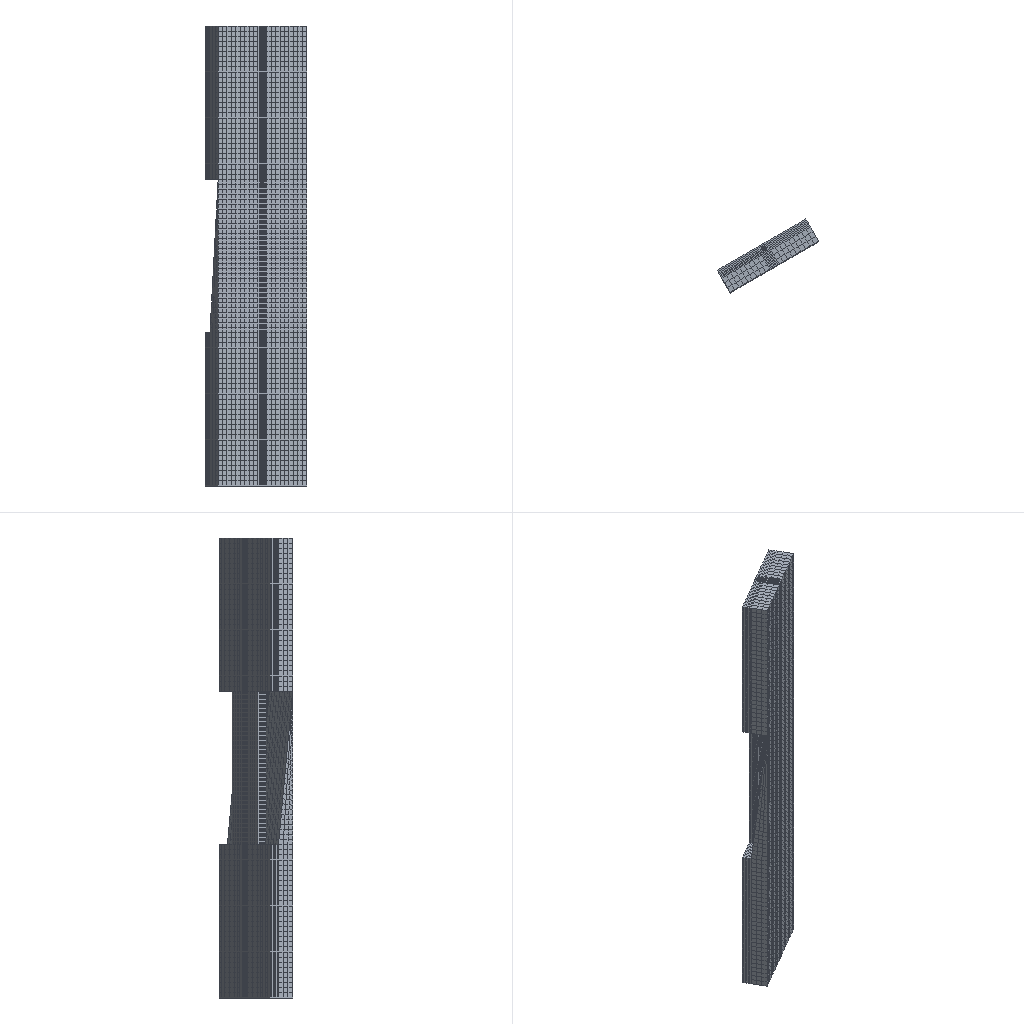Simulation study | abaqus
Set-up summary:
category,name,step,type,value,unit,region
solver,abaqus
solver,version,,,Abaqus/Standard 2020
units,not stated in the deck,,not stated
analysis,deck,,transient,transient
load_step,step,step,transient
load_step,requested,,,1
mesh,nodes,,,35012
mesh,elements,,,27514
element_type,C3D8,,solid,27514
load,load commands in deck,,count,3
bc,support commands in deck,,count,13
material,MAT-HUACHUANG,,in results
material,MAT-PIPE,,in results
material,MATE-HUATI,,in results
check,setup vs results,,match,"per instance, exact: element labels, types and connectivity; labels of the nodes the elements use; coordinates of those nodes at SINGLE_PRECISION in 3 of 3 instance(s)"
Abaqus input file, long lists of numbers shortened:
*Heading
** Job name: Job-2 Model name: Model-1
** Generated by: Abaqus/CAE 2020
*Preprint, echo=NO, model=NO, history=NO, contact=NO
**
** PARTS
**
*Part, name=huachuang
*Node
      1,           5.,   7.59,         120.
      2,           5.,   7.59,         180.
** (21850 more lines like these left out)
*Element, type=C3D8
  1,  2430,  2431, 12315, 12228,    96,    97,  2257,  2256
  2,  2431,  2432, 12316, 12315,    97,    98,  2258,  2257
** (17672 more lines like these left out)
*Nset, nset=Set-9, generate
     1,  21852,      1
*Elset, elset=Set-9, generate
     1,  17674,      1
*Elset, elset=_Surf-huachuang_S4, internal
 9200, 9203, 9206, 9209, 9212, 9215, 9218, 9221, 9224, 9227, 9230, 9233, 9236, 9239, 9242, 9245
 9248, 9251, 9254, 9257, 9260, 9263, 9266, 9269, 9272, 9275, 9278, 9281, 9284, 9287, 9500, 9503
** (1 more lines like these left out)
*Elset, elset=_Surf-huachuang_S3, internal
 9288, 9289, 9290, 9291, 9292, 9293, 9294, 9295, 9296, 9297, 9298, 9299, 9300, 9301, 9302, 9333
 9334, 9335, 9336, 9337, 9338, 9339, 9340, 9341, 9342, 9343, 9344, 9345, 9346, 9347, 9543, 9544
** (1 more lines like these left out)
*Elset, elset=_Surf-huachuang_S2, internal
  4938,  4939,  4940,  4941,  4942,  4943,  4944,  4945,  4946,  4947,  4948,  4949,  4950,  4951,  4952,  4953
  4954,  4955,  4956,  4957,  4958,  4959,  4960,  4961,  4962,  4963,  4964,  4965,  4966,  4967,  4968,  4969
** (15 more lines like these left out)
*Elset, elset=_Surf-huachuang_S5, internal
 12494, 12495, 12496, 12497, 12498, 12499, 12500, 12501, 12502, 12503, 12504, 12505, 12506, 12507, 12508, 12509
 12510, 12511, 12512, 12513, 12514, 12515, 12516, 12517, 12518, 12519, 12520, 12521, 12522, 12523, 12614, 12615
** (15 more lines like these left out)
*Surface, type=ELEMENT, name=Surf-huachuang
_Surf-huachuang_S4, S4
_Surf-huachuang_S3, S3
_Surf-huachuang_S2, S2
_Surf-huachuang_S5, S5
** Section: Section-huachuang
*Solid Section, elset=Set-9, material=Mat-huachuang
,
*End Part
**
*Part, name=huati
*Node
      1,           7.,          10.,         120.
      2,           7.,   8.2,         120.
** (11222 more lines like these left out)
*Element, type=C3D8
  1, 1393, 1394, 6416, 6387,   66,   67, 1268, 1267
  2, 1394, 1395, 6415, 6416,   67,   68, 1269, 1268
** (8878 more lines like these left out)
*Nset, nset=Set-23, generate
     1,  11224,      1
*Elset, elset=Set-23, generate
    1,  8880,     1
** Section: Section-huati
*Solid Section, elset=Set-23, material=Mate-huati
,
*End Part
**
*Part, name=pipe
*Node
      1,  0.5911,           0.,           0.
      2,  0.5911,           0.,         180.
** (1934 more lines like these left out)
*Element, type=C3D8
  1,    8,  377, 1104,  498,    1,   19,  985,  258
  2,  377,  376, 1105, 1104,   19,   20,  986,  985
** (958 more lines like these left out)
*Nset, nset=Set-pipe, generate
    1,  1936,     1
*Elset, elset=Set-pipe, generate
   1,  960,    1
** Section: Section-pipe
*Solid Section, elset=Set-pipe, material=Mat-pipe
,
*End Part
**
**
** ASSEMBLY
**
*Assembly, name=Assembly
**
*Instance, name=huachuang-1, part=huachuang
          0.,           0.,           0.
          0.,           0.,           0.,           0.,           0., 1., 30.
*End Instance
**
*Instance, name=pipe-1, part=pipe
0.2301, 9.601,           0.
0.2301, 9.601,           0., 0.2301, 9.601, 1., 30.
*End Instance
**
*Instance, name=huati-1, part=huati
          0.,           0.,           0.
          0.,           0.,           0.,           0.,           0., 1., 30.
*End Instance
**
*Nset, nset=Set-9, instance=pipe-1, generate
    1,  1936,     1
*Elset, elset=Set-9, instance=pipe-1, generate
   1,  960,    1
*Nset, nset=Set-Huati, instance=huati-1, generate
     1,  11224,      1
*Elset, elset=Set-Huati, instance=huati-1, generate
    1,  8880,     1
*Nset, nset=Set-Huati-Side, instance=huati-1
    1,    2,    3,    4,    5,    6,    7,    8,    9,   10,   11,   12,   13,   14,   15,   16
   17,   18,   19,   20,   21,   22,   23,   24,   25,   26,   27,   28,   29,   30,   31,   32
** (21 more lines like these left out)
*Elset, elset=Set-Huati-Side, instance=huati-1
   30,   31,   32,  120,  150,  151,  181,  182,  183,  271,  272,  273,  274,  275,  276,  451
  452,  453,  454,  571,  572,  573,  661,  662,  663,  664,  781,  782,  783,  784,  785,  786
** (17 more lines like these left out)
*Nset, nset=Set-cemian, instance=huachuang-1
     2,     3,     5,     8,    10,    12,    14,    19,    20,    21,    22,    23,    25,    27,    31,    32
    34,    37,    38,    40,    43,    44,    46,    48,    51,    52,    54,    55,    59,    60,    64,    65
** (36 more lines like these left out)
*Nset, nset=Set-cemian, instance=pipe-1
   1,   2,   3,   4,   5,   6,   7,   8,   9,  10,  11,  12,  13,  14,  15,  16
  17,  18, 138, 258, 378, 498, 618, 619, 739, 740, 741, 861, 862, 982, 983, 984
*Elset, elset=Set-cemian, instance=huachuang-1
   105,   120,   135,   150,   165,   180,   181,   182,   211,   212,   315,   330,   345,   420,   465,   480
   568,   569,   570,   658,   659,   660,   748,   749,   750,   838,   839,   840,  1284,  1285,  1286,  1374
** (30 more lines like these left out)
*Elset, elset=Set-cemian, instance=pipe-1
   1, 120, 121, 240, 241, 360, 361, 480, 481, 600, 601, 720, 721, 840, 841, 960
*Nset, nset=Set-dimian, instance=huachuang-1
    11,    12,    13,    14,    16,    18,    19,    21,    39,    40,    42,    43,    53,    54,    70,    71
    80,    81,    88,    89,   270,   271,   272,   273,   274,   275,   276,   277,   278,   279,   280,   281
** (154 more lines like these left out)
*Elset, elset=Set-dimian, instance=huachuang-1
   481,   484,   487,   490,   493,   496,   499,   502,   505,   508,   511,   514,   517,   520,   523,   526
   529,   532,   535,   538,   541,   544,   547,   550,   553,   556,   559,   562,   565,   568,   571,   574
** (146 more lines like these left out)
*Nset, nset=Set-load, instance=huati-1
   11,   12,   15,   16,   35,   36,  358,  359,  360,  361,  362,  363,  364,  365,  366,  367
  368,  369,  370,  371,  372,  373,  374,  375,  376,  377,  378,  379,  380,  381,  382,  383
** (29 more lines like these left out)
*Elset, elset=Set-load, instance=huati-1
  961,  962,  963,  964,  965,  966,  967,  968,  969,  970,  971,  972,  973,  974,  975,  976
  977,  978,  979,  980,  981,  982,  983,  984,  985,  986,  987,  988,  989,  990,  991,  992
** (25 more lines like these left out)
*Nset, nset=Set-qianmian, instance=huachuang-1
    35,    36,    37,    38,    39,    40,    41,    42,    43,    44,    45,    46,    47,    48,    50,    52
    78,    79,    80,    81,    82,    83,    84,    85,    86,    87,    88,    89,    90,    91,    92,    93
** (93 more lines like these left out)
*Elset, elset=Set-qianmian, instance=huachuang-1
  2517,  2518,  2519,  2520,  2521,  2522,  2523,  2524,  2525,  2526,  2527,  2528,  2529,  2530,  2531,  2532
  2533,  2534,  2535,  2536,  2537,  2538,  2539,  2540,  2541,  2542,  2543,  2544,  2545,  2546,  2547,  2548
** (79 more lines like these left out)
*Nset, nset=huachuang, instance=huachuang-1
     1,     2,     3,     4,     5,     6,     7,     8,     9,    10,    11,    12,    13,    14,    15,    16
    17,    18,    19,    20,    21,    22,    23,    24,    25,    26,    27,    28,    29,    30,    31,    32
** (1269 more lines like these left out)
*Elset, elset=huachuang, instance=huachuang-1
     1,     2,     3,     4,     5,     6,     7,     8,     9,    10,    11,    12,    13,    14,    15,    16
    17,    18,    19,    20,    21,    22,    23,    24,    25,    26,    27,    28,    29,    30,    31,    32
** (1031 more lines like these left out)
*Nset, nset=model-all, instance=huachuang-1
     1,     2,     3,     4,     5,     6,     7,     8,     9,    10,    11,    12,    13,    14,    15,    16
    17,    18,    19,    20,    21,    22,    23,    24,    25,    26,    27,    28,    29,    30,    31,    32
** (1269 more lines like these left out)
*Nset, nset=model-all, instance=pipe-1, generate
    1,  1936,     1
*Nset, nset=model-all, instance=huati-1, generate
     1,  11224,      1
*Elset, elset=model-all, instance=huachuang-1
     1,     2,     3,     4,     5,     6,     7,     8,     9,    10,    11,    12,    13,    14,    15,    16
    17,    18,    19,    20,    21,    22,    23,    24,    25,    26,    27,    28,    29,    30,    31,    32
** (1031 more lines like these left out)
*Elset, elset=model-all, instance=pipe-1, generate
   1,  960,    1
*Elset, elset=model-all, instance=huati-1, generate
    1,  8880,     1
*Elset, elset=_Huachuang-mid-top_S4, internal, instance=huachuang-1
  1602,  1603,  1604,  1605,  1606,  1607,  1608,  1609,  1610,  1611,  1612,  1613,  1614,  1615,  1616,  1617
  1618,  1619,  1620,  1621,  1622,  1623,  1624,  1625,  1626,  1627,  1628,  1629,  1630,  1631,  1632,  1633
** (21 more lines like these left out)
*Elset, elset=_Huachuang-mid-top_S2, internal, instance=huachuang-1
  1827,  1828,  1829,  1830,  1831,  1832,  1833,  1834,  1835,  1836,  1837,  1838,  1839,  1840,  1841,  1842
  1843,  1844,  1845,  1846,  1847,  1848,  1849,  1850,  1851,  1852,  1853,  1854,  1855,  1856, 15905, 15906
** (19 more lines like these left out)
*Elset, elset=_Huachuang-mid-top_S3, internal, instance=huachuang-1
  1557,  1558,  1559,  1560,  1561,  1562,  1563,  1564,  1565,  1566,  1567,  1568,  1569,  1570,  1571,  1572
  1573,  1574,  1575,  1576,  1577,  1578,  1579,  1580,  1581,  1582,  1583,  1584,  1585,  1586,  1587,  1588
** (4 more lines like these left out)
*Surface, type=ELEMENT, name=Huachuang-mid-top
_Huachuang-mid-top_S4, S4
_Huachuang-mid-top_S2, S2
_Huachuang-mid-top_S3, S3
*Elset, elset=_Huati-bottom_S2, internal, instance=huati-1
  961,  962,  963,  964,  965,  966,  967,  968,  969,  970,  971,  972,  973,  974,  975,  976
  977,  978,  979,  980,  981,  982,  983,  984,  985,  986,  987,  988,  989,  990,  991,  992
** (43 more lines like these left out)
*Elset, elset=_Huati-bottom_S3, internal, instance=huati-1
 5101, 5102, 5103, 5104, 5105, 5106, 5107, 5108, 5109, 5110, 5111, 5112, 5113, 5114, 5115, 5116
 5117, 5118, 5119, 5120, 5121, 5122, 5123, 5124, 5125, 5126, 5127, 5128, 5129, 5130, 5131, 5132
** (10 more lines like these left out)
*Elset, elset=_Huati-bottom_S4, internal, instance=huati-1
 4801, 4802, 4803, 4804, 4805, 4806, 4807, 4808, 4809, 4810, 4811, 4812, 4813, 4814, 4815, 4816
 4817, 4818, 4819, 4820, 4821, 4822, 4823, 4824, 4825, 4826, 4827, 4828, 4829, 4830, 4831, 4832
** (10 more lines like these left out)
*Surface, type=ELEMENT, name=Huati-bottom
_Huati-bottom_S2, S2
_Huati-bottom_S3, S3
_Huati-bottom_S4, S4
*Elset, elset=_Surf-13_S2, internal, instance=pipe-1
   1,   2,   3,   4,   5,   6,   7,   8,   9,  10,  11,  12,  13,  14,  15,  16
  17,  18,  19,  20,  21,  22,  23,  24,  25,  26,  27,  28,  29,  30,  31,  32
** (28 more lines like these left out)
*Surface, type=ELEMENT, name=Surf-13
_Surf-13_S2, S2
*Elset, elset=_Surf-LOAD_S3, internal, instance=huati-1
  961,  962,  963,  964,  965,  966,  967,  968,  969,  970,  971,  972,  973,  974,  975,  976
  977,  978,  979,  980,  981,  982,  983,  984,  985,  986,  987,  988,  989,  990,  991,  992
** (25 more lines like these left out)
*Surface, type=ELEMENT, name=Surf-LOAD
_Surf-LOAD_S3, S3
*Elset, elset=_Surf-huachuang_S3, internal, instance=huachuang-1
  1647,  1648,  1649,  1650,  1651,  1652,  1653,  1654,  1655,  1656,  1657,  1658,  1659,  1660,  1661,  1677
  1678,  1679,  1680,  1681,  1682,  1683,  1684,  1685,  1686,  1687,  1688,  1689,  1690,  1691,  1707,  1708
** (27 more lines like these left out)
*Elset, elset=_Surf-huachuang_S4, internal, instance=huachuang-1
  1738,  1740,  1742,  1744,  1746,  1748,  1750,  1752,  1754,  1756,  1758,  1760,  1762,  1764,  1766,  1768
  1770,  1772,  1774,  1776,  1778,  1780,  1782,  1784,  1786,  1788,  1790,  1792,  1794,  1796,  1798,  1800
** (24 more lines like these left out)
*Elset, elset=_Surf-huachuang_S2, internal, instance=huachuang-1
     1,     2,     3,     4,     5,     6,     7,     8,     9,    10,    11,    12,    13,    14,    15,    16
    17,    18,    19,    20,    21,    22,    23,    24,    25,    26,    27,    28,    29,    30,    31,    32
** (22 more lines like these left out)
*Surface, type=ELEMENT, name=Surf-huachuang
_Surf-huachuang_S3, S3
_Surf-huachuang_S4, S4
_Surf-huachuang_S2, S2
*Elset, elset=_Surf-huati_S3, internal, instance=huati-1
  451,  452,  455,  456,  459,  460,  463,  464,  467,  468,  471,  472,  475,  476,  479,  480
  483,  484,  487,  488,  491,  492,  495,  496,  499,  500,  503,  504,  507,  508,  511,  512
** (42 more lines like these left out)
*Elset, elset=_Surf-huati_S4, internal, instance=huati-1
  272,  274,  276,  278,  280,  282,  284,  286,  288,  290,  292,  294,  296,  298,  300,  302
  304,  306,  308,  310,  312,  314,  316,  318,  320,  322,  324,  326,  328,  330,  332,  334
** (30 more lines like these left out)
*Surface, type=ELEMENT, name=Surf-huati
_Surf-huati_S3, S3
_Surf-huati_S4, S4
*Elset, elset=_Surf-pipe_S1, internal, instance=pipe-1, generate
   1,  960,    1
*Surface, type=ELEMENT, name=Surf-pipe
_Surf-pipe_S1, S1
*Elset, elset=_huachuang-left-side_S2, internal, instance=huachuang-1
  7368,  7369,  7370,  7371,  7372,  7373,  7374,  7375,  7376,  7377,  7378,  7379,  7380,  7381,  7382,  7383
  7384,  7385,  7386,  7387,  7388,  7389,  7390,  7391,  7392,  7393,  7394,  8808,  8809,  8810,  8811,  8868
** (2 more lines like these left out)
*Elset, elset=_huachuang-left-side_S3, internal, instance=huachuang-1
    1,    2,    3,   46,   47,   48,  346,  361,  376,  391,  421,  422, 2517, 2518, 2519, 2607
 2608, 2609, 2697, 2698, 2699, 2787, 2788, 2789, 2877, 2878, 2879, 2967, 2968, 2969, 3057, 3058
** (1 more lines like these left out)
*Elset, elset=_huachuang-left-side_S4, internal, instance=huachuang-1
  255,  270,  285,  300, 8552, 8567, 8582, 8597, 8612, 8627, 9122, 9137, 9152, 9167, 9182, 9197
 9437, 9452, 9467, 9497, 9557, 9572, 9587
*Elset, elset=_huachuang-left-side_S6, internal, instance=huachuang-1, generate
 11594,  13454,     30
*Surface, type=ELEMENT, name=huachuang-left-side
_huachuang-left-side_S2, S2
_huachuang-left-side_S3, S3
_huachuang-left-side_S4, S4
_huachuang-left-side_S6, S6
*Elset, elset=_huachuang-right-side_S3, internal, instance=huachuang-1
  1737,  1738,  1767,  1768,  1797,  1798,  2037,  2052,  2067,  5748,  5749,  5750,  5838,  5839,  5840,  5928
  5929,  5930,  6018,  6019,  6020,  6108,  6109,  6110,  6198,  6199,  6200,  6288,  6289,  6290,  6378,  6379
** (5 more lines like these left out)
*Elset, elset=_huachuang-right-side_S4, internal, instance=huachuang-1
  1571,  1586,  1601,  1856,  1901,  1916,  1991,  2006,  2021,  2036,  2096,  2111,  2126,  2141,  2156,  2171
 10318, 10333, 10348, 15934, 15964, 15994, 16024, 16054, 16084, 16114, 16144, 16174, 16204, 16234, 16264, 16294
** (2 more lines like these left out)
*Elset, elset=_huachuang-right-side_S2, internal, instance=huachuang-1
  2307,  2308,  2309,  2310,  2367,  2368,  2397, 10574, 10589, 10590, 10619, 10620, 10621, 10622
*Surface, type=ELEMENT, name=huachuang-right-side
_huachuang-right-side_S3, S3
_huachuang-right-side_S4, S4
_huachuang-right-side_S2, S2
*Elset, elset=_huati-left-side_S4, internal, instance=huati-1
   30, 1020, 1080, 1140, 1200, 1260, 1320, 1380, 1440, 1500, 1560, 1620, 1680, 1740, 1800, 1860
 1920, 1980, 2040, 2100, 2160, 2220, 2280, 2340, 2400, 3960, 3990, 5130, 5160, 5490, 5520, 5550
** (2 more lines like these left out)
*Elset, elset=_huati-left-side_S3, internal, instance=huati-1
   31,   32, 3991, 4411, 4412, 4413, 4981, 4982, 5041, 5042, 5551, 8221, 8251, 8611, 8612, 8613
*Elset, elset=_huati-left-side_S2, internal, instance=huati-1
  181,  182,  183,  271,  272,  273,  274,  275,  276,  451,  452,  453,  454, 4501, 4502, 4503
 4504, 4621, 4622, 4623, 4624, 4625, 4626, 8701, 8702, 8703, 8704, 8705, 8706
*Elset, elset=_huati-left-side_S6, internal, instance=huati-1
 2401, 2461, 2521, 2581, 2641, 2701, 2761, 2821, 2881, 2941, 3001, 3061, 3121, 3181, 3241, 3301
 3361, 3421, 3481, 3541, 3601, 3661, 3721, 3781, 6841, 6901, 6961, 7021, 7081, 7141, 7201, 7261
** (1 more lines like these left out)
*Surface, type=ELEMENT, name=huati-left-side
_huati-left-side_S4, S4
_huati-left-side_S3, S3
_huati-left-side_S2, S2
_huati-left-side_S6, S6
*Elset, elset=_huati-right-side_S4, internal, instance=huati-1
  120,  150, 2460, 2520, 2580, 2640, 2700, 2760, 2820, 2880, 2940, 3000, 3060, 3120, 3180, 3240
 3300, 3360, 3420, 3480, 3540, 3600, 3660, 3720, 3780, 3840, 3870, 4890, 4920, 4950, 4980, 6900
** (2 more lines like these left out)
*Elset, elset=_huati-right-side_S6, internal, instance=huati-1
  961, 1021, 1081, 1141, 1201, 1261, 1321, 1381, 1441, 1501, 1561, 1621, 1681, 1741, 1801, 1861
 1921, 1981, 2041, 2101, 2161, 2221, 2281, 2341, 5761, 5821, 5881, 5941, 6001, 6061, 6121, 6181
** (1 more lines like these left out)
*Elset, elset=_huati-right-side_S3, internal, instance=huati-1
  151,  571,  572,  573, 3871, 3872, 4801, 4831, 7981, 7982, 8041, 8042
*Elset, elset=_huati-right-side_S2, internal, instance=huati-1
  661,  662,  663,  664,  781,  782,  783,  784,  785,  786, 4021, 4022, 4023, 4111, 4112, 4113
 4114, 4115, 4116, 4291, 4292, 4293, 4294, 5161, 5162, 5163, 5164, 5165, 5166, 5341, 5342, 5343
** (1 more lines like these left out)
*Surface, type=ELEMENT, name=huati-right-side
_huati-right-side_S4, S4
_huati-right-side_S6, S6
_huati-right-side_S2, S2
_huati-right-side_S3, S3
*Elset, elset=_m_Surf-15_S3, internal, instance=huachuang-1
  1557,  1558,  1559,  1560,  1561,  1562,  1563,  1564,  1565,  1566,  1567,  1568,  1569,  1570,  1571,  1572
  1573,  1574,  1575,  1576,  1577,  1578,  1579,  1580,  1581,  1582,  1583,  1584,  1585,  1586,  1587,  1588
** (4 more lines like these left out)
*Elset, elset=_m_Surf-15_S3, internal, instance=huati-1
 5101, 5102, 5103, 5104, 5105, 5106, 5107, 5108, 5109, 5110, 5111, 5112, 5113, 5114, 5115, 5116
 5117, 5118, 5119, 5120, 5121, 5122, 5123, 5124, 5125, 5126, 5127, 5128, 5129, 5130, 5131, 5132
** (10 more lines like these left out)
*Elset, elset=_m_Surf-15_S4, internal, instance=huachuang-1
  1602,  1603,  1604,  1605,  1606,  1607,  1608,  1609,  1610,  1611,  1612,  1613,  1614,  1615,  1616,  1617
  1618,  1619,  1620,  1621,  1622,  1623,  1624,  1625,  1626,  1627,  1628,  1629,  1630,  1631,  1632,  1633
** (21 more lines like these left out)
*Elset, elset=_m_Surf-15_S4, internal, instance=huati-1
 4801, 4802, 4803, 4804, 4805, 4806, 4807, 4808, 4809, 4810, 4811, 4812, 4813, 4814, 4815, 4816
 4817, 4818, 4819, 4820, 4821, 4822, 4823, 4824, 4825, 4826, 4827, 4828, 4829, 4830, 4831, 4832
** (10 more lines like these left out)
*Elset, elset=_m_Surf-15_S2, internal, instance=huachuang-1
  1827,  1828,  1829,  1830,  1831,  1832,  1833,  1834,  1835,  1836,  1837,  1838,  1839,  1840,  1841,  1842
  1843,  1844,  1845,  1846,  1847,  1848,  1849,  1850,  1851,  1852,  1853,  1854,  1855,  1856, 15905, 15906
** (19 more lines like these left out)
*Elset, elset=_m_Surf-15_S2, internal, instance=huati-1
  961,  962,  963,  964,  965,  966,  967,  968,  969,  970,  971,  972,  973,  974,  975,  976
  977,  978,  979,  980,  981,  982,  983,  984,  985,  986,  987,  988,  989,  990,  991,  992
** (43 more lines like these left out)
*Surface, type=ELEMENT, name=m_Surf-15
_m_Surf-15_S3, S3
_m_Surf-15_S4, S4
_m_Surf-15_S2, S2
*Elset, elset=_m_Surf-16_S2, internal, instance=huati-1
  961,  962,  963,  964,  965,  966,  967,  968,  969,  970,  971,  972,  973,  974,  975,  976
  977,  978,  979,  980,  981,  982,  983,  984,  985,  986,  987,  988,  989,  990,  991,  992
** (43 more lines like these left out)
*Elset, elset=_m_Surf-16_S3, internal, instance=huati-1
 5101, 5102, 5103, 5104, 5105, 5106, 5107, 5108, 5109, 5110, 5111, 5112, 5113, 5114, 5115, 5116
 5117, 5118, 5119, 5120, 5121, 5122, 5123, 5124, 5125, 5126, 5127, 5128, 5129, 5130, 5131, 5132
** (10 more lines like these left out)
*Elset, elset=_m_Surf-16_S4, internal, instance=huati-1
 4801, 4802, 4803, 4804, 4805, 4806, 4807, 4808, 4809, 4810, 4811, 4812, 4813, 4814, 4815, 4816
 4817, 4818, 4819, 4820, 4821, 4822, 4823, 4824, 4825, 4826, 4827, 4828, 4829, 4830, 4831, 4832
** (10 more lines like these left out)
*Surface, type=ELEMENT, name=m_Surf-16
_m_Surf-16_S2, S2
_m_Surf-16_S3, S3
_m_Surf-16_S4, S4
*Elset, elset=_pipe-inner_S2, internal, instance=pipe-1, generate
   1,  960,    1
*Surface, type=ELEMENT, name=pipe-inner
_pipe-inner_S2, S2
*Elset, elset=_s_Surf-14_S4, internal, instance=huachuang-1
   958,   960,  4138,  4140,  4142,  4144,  4146,  4148,  4150,  4152,  4154,  4156,  4158,  4160,  4162,  4164
  4166,  4168,  4170,  4172,  4174,  4176,  4178,  4180,  4182,  4184,  4186,  4188,  4190,  4192,  4194,  4196
** (26 more lines like these left out)
*Elset, elset=_s_Surf-14_S3, internal, instance=huachuang-1
   841,   842,   843,   844,   845,   846,   847,   848,   849,   850,   851,   852,   853,   854,   855,   856
   857,   858,   859,   860,   861,   862,   863,   864,   865,   866,   867,   868,   869,   899,   900,   901
** (3 more lines like these left out)
*Elset, elset=_s_Surf-14_S2, internal, instance=huachuang-1
  1019,  1020,  1023,  1024,  1025,  1026,  1027,  1028,  1029,  1030,  1031,  1032,  1033,  1034,  1035,  1036
  1037,  1038,  1039,  1040,  1041,  1042,  1043,  1044,  1045,  1046,  1047,  1048,  1049,  1050,  1051,  1052
** (15 more lines like these left out)
*Surface, type=ELEMENT, name=s_Surf-14
_s_Surf-14_S4, S4
_s_Surf-14_S3, S3
_s_Surf-14_S2, S2
*End Assembly
*Amplitude, name=Amp-1
             0.,              0.,              1.,              1.
**
** MATERIALS
**
*Material, name=Mat-huachuang
*Density
1800.,
*Elastic
 3.2e+06, 0.28
*Mohr Coulomb
20., 0.1
*Mohr Coulomb Hardening
 2e+07,0.
*Material, name=Mat-pipe
*Density
7900.,
*Elastic
 2.1e+11, 0.3
*Expansion
 1.25e-05,
*Plastic
 4.60095e+08,          0.
 4.67441e+08,    8.87e-06
 4.74118e+08,    1.63e-05
 4.80796e+08,    2.73e-05
 4.87474e+08,    4.35e-05
 4.94152e+08,    6.72e-05
 5.00829e+08, 0.0001015
 5.07507e+08, 0.000151
 5.14185e+08,   0.0002218
 5.20862e+08, 0.0003226
  5.2754e+08, 0.000465
 5.34218e+08, 0.0006646
 5.40896e+08, 0.0009423
 5.47573e+08,  0.001325
 5.54251e+08,   0.001846
 5.60929e+08,  0.002547
 5.67607e+08,  0.003475
 5.74284e+08,  0.004684
 5.80962e+08,  0.006226
  5.8764e+08,  0.008154
 5.94317e+08,   0.01051
 6.00995e+08,   0.01331
 6.07673e+08,   0.01658
 6.14351e+08,   0.02031
 6.21028e+08,   0.02448
 6.27706e+08,   0.02906
 6.34384e+08,   0.03401
 6.41061e+08,   0.03929
 6.47739e+08,   0.04486
 6.54417e+08,   0.05071
 6.61095e+08,   0.05683
 6.67772e+08,   0.06302
*Material, name=Mate-huati
*Density
1800.,
*Elastic
 3.115e+06, 0.3
*Mohr Coulomb
20., 0.1
*Mohr Coulomb Hardening
 2e+07,0.
**
** INTERACTION PROPERTIES
**
*Surface Interaction, name=IntProp-1
1.,
*Friction, slip tolerance=0.005
 0.3,
*Surface Behavior, penalty=NONLINEAR
*Surface Interaction, name=IntProp-1-Copy
1.,
*Friction, slip tolerance=0.005
 0.3,
*Surface Behavior, pressure-overclosure=HARD
**
** BOUNDARY CONDITIONS
**
** Name: huachuang-cemian Type: Displacement/rotation angle
*Boundary
Set-cemian, 1, 1
Set-cemian, 3, 3
** Name: huachuang-dimian Type: Displacement/rotation angle
*Boundary
Set-dimian, 1, 1
Set-dimian, 2, 2
Set-dimian, 3, 3
** Name: huachuang-qianmian Type: Displacement/rotation angle
*Boundary
Set-qianmian, 1, 1
** Name: huati-beimian Type: Displacement/rotation angle
*Boundary
Set-load, 1, 1
**
** PREDEFINED FIELDS
**
** Name: Predefined Field-1   Type: Temperature
*Initial Conditions, type=TEMPERATURE
Set-9, 0.
**
** INTERACTIONS
**
** Interaction: Huachuang-Huati
*Contact Pair, interaction=IntProp-1-Copy, type=SURFACE TO SURFACE
s_Surf-14, m_Surf-16
** Interaction: huachuang-huati-left-side
*Contact Pair, interaction=IntProp-1-Copy, type=SURFACE TO SURFACE
huati-left-side, huachuang-left-side
** Interaction: huachuang-huati-right-side
*Contact Pair, interaction=IntProp-1-Copy, type=SURFACE TO SURFACE
huati-right-side, huachuang-right-side
** Interaction: pipe-huachuang
*Contact Pair, interaction=IntProp-1-Copy, type=SURFACE TO SURFACE
Surf-huachuang, Surf-pipe
** Interaction: pipe-huati
*Contact Pair, interaction=IntProp-1-Copy, type=SURFACE TO SURFACE
Surf-huati, Surf-pipe
** ----------------------------------------------------------------
**
** STEP: step
**
*Step, name=step, nlgeom=YES, inc=10000, unsymm=YES
*Dynamic
0.001,1.,1e-05
**
** BOUNDARY CONDITIONS
**
** Name: huachuang-cemian Type: Displacement/rotation angle
*Boundary, op=NEW
Set-cemian, 1, 1
Set-cemian, 3, 3
** Name: huachuang-dimian Type: Displacement/rotation angle
*Boundary, op=NEW
Set-dimian, 1, 1
Set-dimian, 2, 2
Set-dimian, 3, 3
** Name: huachuang-qianmian Type: Displacement/rotation angle
*Boundary, op=NEW
Set-qianmian, 1, 1
** Name: huati-beimian Type: Displacement/rotation angle
*Boundary, op=NEW
**
** LOADS
**
** Name: Gravity   Type: Gravity
*Dload
model-all, GRAV, 9.8, 0., -1., 0.
** Name: Load-3   Type: Pressure
*Dsload, amplitude=Amp-1
Surf-13, P, 100000.
**
** PREDEFINED FIELDS
**
** Name: Predefined Field-1   Type: Temperature
*Temperature
Set-9, 30.
**
** CONTROLS
**
*Controls, reset
*Controls, parameters=time incrementation
, 20, , , , , , 20, , ,
**
** OUTPUT REQUESTS
**
*Restart, write, frequency=0
**
** FIELD OUTPUT: F-Output-1
**
*Output, field, frequency=1
*Node Output
CF, NT, RF, RM, RT, U
*Element Output, directions=YES
LE, NFORC, PE, PEEQ, PEMAG, S, TEMP
*Contact Output
CDISP, CSTRESS
*Output, history, frequency=0
*End Step
Results summary:
result,step,,completed,increments=38 time=1.0/1.0
result,analysis,,,transient
result,last_loadstep,,,1
result,primary field,,,U
result,reaction total,,FX,47997381.713,model units
result,reaction total,,FY,852664543.008,model units
result,reaction total,,FZ,28705670.862,model units